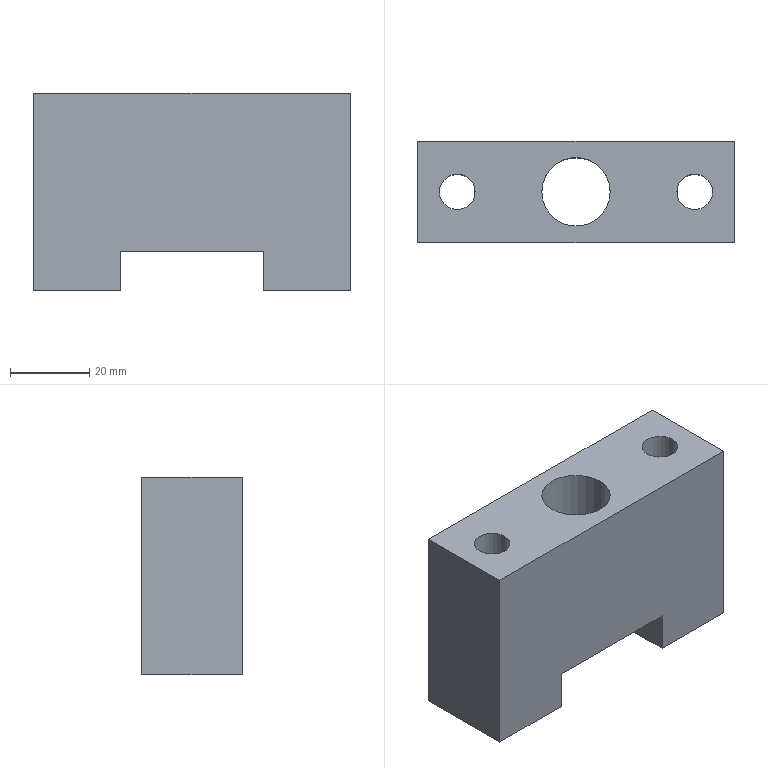Part | STEP file | giu lo xo day chot xien | 1 solid | 16 faces | box 80 x 25.5 x 50 mm | volume 77062 mm3 | plane 10 | cylinder 6 | commonest cylinder face diameters 9 x4 17.294 x2
STEP:
#1=CARTESIAN_POINT('',(0.,0.,0.));
#2=DIRECTION('',(0.,0.,1.));
#3=DIRECTION('',(1.,0.,0.));
#4=AXIS2_PLACEMENT_3D('',#1,#2,#3);
#5=CARTESIAN_POINT('',(14.5,12.75,0.));
#6=VERTEX_POINT('',#5);
#7=CARTESIAN_POINT('',(14.5,12.75,50.));
#8=VERTEX_POINT('',#7);
#9=CARTESIAN_POINT('',(14.5,12.75,-47.725));
#10=DIRECTION('',(0.,0.,1.));
#11=VECTOR('',#10,1.);
#12=LINE('',#9,#11);
#13=CARTESIAN_POINT('',(10.,12.75,-47.725));
#14=DIRECTION('',(0.,0.,1.));
#15=DIRECTION('',(1.,0.,0.));
#16=AXIS2_PLACEMENT_3D('',#13,#14,#15);
#17=CYLINDRICAL_SURFACE('',#16,4.5);
#18=CARTESIAN_POINT('',(6.283,0.));
#19=DIRECTION('',(0.,1.));
#20=VECTOR('',#19,1.);
#21=LINE('',#18,#20);
#22=(GEOMETRIC_REPRESENTATION_CONTEXT(2)PARAMETRIC_REPRESENTATION_CONTEXT()REPRESENTATION_CONTEXT('',''));
#23=DEFINITIONAL_REPRESENTATION('',(#21),#22);
#24=PCURVE('',#17,#23);
#25=CARTESIAN_POINT('',(10.,12.75,-47.725));
#26=DIRECTION('',(0.,0.,1.));
#27=DIRECTION('',(1.,0.,0.));
#28=AXIS2_PLACEMENT_3D('',#25,#26,#27);
#29=CYLINDRICAL_SURFACE('',#28,4.5);
#30=CARTESIAN_POINT('',(0.,0.));
#31=DIRECTION('',(0.,1.));
#32=VECTOR('',#31,1.);
#33=LINE('',#30,#32);
#34=(GEOMETRIC_REPRESENTATION_CONTEXT(2)PARAMETRIC_REPRESENTATION_CONTEXT()REPRESENTATION_CONTEXT('',''));
#35=DEFINITIONAL_REPRESENTATION('',(#33),#34);
#36=PCURVE('',#29,#35);
#37=SURFACE_CURVE('',#12,(#24,#36),.PCURVE_S1.);
#38=EDGE_CURVE('',#6,#8,#37,.T.);
#39=ORIENTED_EDGE('',*,*,#38,.T.);
#40=CARTESIAN_POINT('',(5.5,12.75,50.));
#41=VERTEX_POINT('',#40);
#42=CARTESIAN_POINT('',(10.,12.75,50.));
#43=DIRECTION('',(0.,0.,-1.));
#44=DIRECTION('',(1.,0.,0.));
#45=AXIS2_PLACEMENT_3D('',#42,#43,#44);
#46=CIRCLE('',#45,4.5);
#47=CARTESIAN_POINT('',(6.283,97.725));
#48=DIRECTION('',(-1.,0.));
#49=VECTOR('',#48,1.);
#50=LINE('',#47,#49);
#51=(GEOMETRIC_REPRESENTATION_CONTEXT(2)PARAMETRIC_REPRESENTATION_CONTEXT()REPRESENTATION_CONTEXT('',''));
#52=DEFINITIONAL_REPRESENTATION('',(#50),#51);
#53=PCURVE('',#17,#52);
#54=CARTESIAN_POINT('',(40.,12.75,50.));
#55=DIRECTION('',(0.,0.,1.));
#56=DIRECTION('',(1.,0.,0.));
#57=AXIS2_PLACEMENT_3D('',#54,#55,#56);
#58=PLANE('',#57);
#59=CARTESIAN_POINT('',(-25.5,0.));
#60=CARTESIAN_POINT('',(-25.5,-7.794));
#61=CARTESIAN_POINT('',(-32.25,-3.897));
#62=CARTESIAN_POINT('',(-39.,0.));
#63=CARTESIAN_POINT('',(-32.25,3.897));
#64=CARTESIAN_POINT('',(-25.5,7.794));
#65=CARTESIAN_POINT('',(-25.5,0.));
#66=(BOUNDED_CURVE()B_SPLINE_CURVE(2,(#59,#60,#61,#62,#63,#64,#65),.UNSPECIFIED.,.T.,.F.)B_SPLINE_CURVE_WITH_KNOTS((1,2,2,2,2,1),(-2.094,0.,2.094,4.189,6.283,8.378),.UNSPECIFIED.)CURVE()GEOMETRIC_REPRESENTATION_ITEM()RATIONAL_B_SPLINE_CURVE((1.,0.5,1.,0.5,1.,0.5,1.))REPRESENTATION_ITEM(''));
#67=(GEOMETRIC_REPRESENTATION_CONTEXT(2)PARAMETRIC_REPRESENTATION_CONTEXT()REPRESENTATION_CONTEXT('',''));
#68=DEFINITIONAL_REPRESENTATION('',(#66),#67);
#69=PCURVE('',#58,#68);
#70=SURFACE_CURVE('',#46,(#53,#69),.PCURVE_S1.);
#71=EDGE_CURVE('',#8,#41,#70,.T.);
#72=ORIENTED_EDGE('',*,*,#71,.T.);
#73=CARTESIAN_POINT('',(5.5,12.75,0.));
#74=VERTEX_POINT('',#73);
#75=CARTESIAN_POINT('',(5.5,12.75,-47.725));
#76=DIRECTION('',(0.,0.,1.));
#77=VECTOR('',#76,1.);
#78=LINE('',#75,#77);
#79=CARTESIAN_POINT('',(3.142,0.));
#80=DIRECTION('',(0.,1.));
#81=VECTOR('',#80,1.);
#82=LINE('',#79,#81);
#83=(GEOMETRIC_REPRESENTATION_CONTEXT(2)PARAMETRIC_REPRESENTATION_CONTEXT()REPRESENTATION_CONTEXT('',''));
#84=DEFINITIONAL_REPRESENTATION('',(#82),#83);
#85=PCURVE('',#17,#84);
#86=CARTESIAN_POINT('',(3.142,0.));
#87=DIRECTION('',(0.,1.));
#88=VECTOR('',#87,1.);
#89=LINE('',#86,#88);
#90=(GEOMETRIC_REPRESENTATION_CONTEXT(2)PARAMETRIC_REPRESENTATION_CONTEXT()REPRESENTATION_CONTEXT('',''));
#91=DEFINITIONAL_REPRESENTATION('',(#89),#90);
#92=PCURVE('',#29,#91);
#93=SURFACE_CURVE('',#78,(#85,#92),.PCURVE_S1.);
#94=EDGE_CURVE('',#74,#41,#93,.T.);
#95=ORIENTED_EDGE('',*,*,#94,.F.);
#96=CARTESIAN_POINT('',(10.,12.75,0.));
#97=DIRECTION('',(0.,0.,-1.));
#98=DIRECTION('',(1.,0.,0.));
#99=AXIS2_PLACEMENT_3D('',#96,#97,#98);
#100=CIRCLE('',#99,4.5);
#101=CARTESIAN_POINT('',(6.283,47.725));
#102=DIRECTION('',(-1.,0.));
#103=VECTOR('',#102,1.);
#104=LINE('',#101,#103);
#105=(GEOMETRIC_REPRESENTATION_CONTEXT(2)PARAMETRIC_REPRESENTATION_CONTEXT()REPRESENTATION_CONTEXT('',''));
#106=DEFINITIONAL_REPRESENTATION('',(#104),#105);
#107=PCURVE('',#17,#106);
#108=CARTESIAN_POINT('',(40.,12.75,0.));
#109=DIRECTION('',(0.,0.,1.));
#110=DIRECTION('',(1.,0.,0.));
#111=AXIS2_PLACEMENT_3D('',#108,#109,#110);
#112=PLANE('',#111);
#113=CARTESIAN_POINT('',(-25.5,0.));
#114=CARTESIAN_POINT('',(-25.5,-7.794));
#115=CARTESIAN_POINT('',(-32.25,-3.897));
#116=CARTESIAN_POINT('',(-39.,0.));
#117=CARTESIAN_POINT('',(-32.25,3.897));
#118=CARTESIAN_POINT('',(-25.5,7.794));
#119=CARTESIAN_POINT('',(-25.5,0.));
#120=(BOUNDED_CURVE()B_SPLINE_CURVE(2,(#113,#114,#115,#116,#117,#118,#119),.UNSPECIFIED.,.T.,.F.)B_SPLINE_CURVE_WITH_KNOTS((1,2,2,2,2,1),(-2.094,0.,2.094,4.189,6.283,8.378),.UNSPECIFIED.)CURVE()GEOMETRIC_REPRESENTATION_ITEM()RATIONAL_B_SPLINE_CURVE((1.,0.5,1.,0.5,1.,0.5,1.))REPRESENTATION_ITEM(''));
#121=(GEOMETRIC_REPRESENTATION_CONTEXT(2)PARAMETRIC_REPRESENTATION_CONTEXT()REPRESENTATION_CONTEXT('',''));
#122=DEFINITIONAL_REPRESENTATION('',(#120),#121);
#123=PCURVE('',#112,#122);
#124=SURFACE_CURVE('',#100,(#107,#123),.PCURVE_S1.);
#125=EDGE_CURVE('',#6,#74,#124,.T.);
#126=ORIENTED_EDGE('',*,*,#125,.F.);
#127=EDGE_LOOP('',(#39,#72,#95,#126));
#128=FACE_BOUND('',#127,.F.);
#129=ADVANCED_FACE('',(#128),#17,.F.);
#130=CARTESIAN_POINT('',(74.5,12.75,0.));
#131=VERTEX_POINT('',#130);
#132=CARTESIAN_POINT('',(74.5,12.75,50.));
#133=VERTEX_POINT('',#132);
#134=CARTESIAN_POINT('',(74.5,12.75,-47.725));
#135=DIRECTION('',(0.,0.,1.));
#136=VECTOR('',#135,1.);
#137=LINE('',#134,#136);
#138=CARTESIAN_POINT('',(70.,12.75,-47.725));
#139=DIRECTION('',(0.,0.,1.));
#140=DIRECTION('',(1.,0.,0.));
#141=AXIS2_PLACEMENT_3D('',#138,#139,#140);
#142=CYLINDRICAL_SURFACE('',#141,4.5);
#143=CARTESIAN_POINT('',(6.283,0.));
#144=DIRECTION('',(0.,1.));
#145=VECTOR('',#144,1.);
#146=LINE('',#143,#145);
#147=(GEOMETRIC_REPRESENTATION_CONTEXT(2)PARAMETRIC_REPRESENTATION_CONTEXT()REPRESENTATION_CONTEXT('',''));
#148=DEFINITIONAL_REPRESENTATION('',(#146),#147);
#149=PCURVE('',#142,#148);
#150=CARTESIAN_POINT('',(70.,12.75,-47.725));
#151=DIRECTION('',(0.,0.,1.));
#152=DIRECTION('',(1.,0.,0.));
#153=AXIS2_PLACEMENT_3D('',#150,#151,#152);
#154=CYLINDRICAL_SURFACE('',#153,4.5);
#155=CARTESIAN_POINT('',(0.,0.));
#156=DIRECTION('',(0.,1.));
#157=VECTOR('',#156,1.);
#158=LINE('',#155,#157);
#159=(GEOMETRIC_REPRESENTATION_CONTEXT(2)PARAMETRIC_REPRESENTATION_CONTEXT()REPRESENTATION_CONTEXT('',''));
#160=DEFINITIONAL_REPRESENTATION('',(#158),#159);
#161=PCURVE('',#154,#160);
#162=SURFACE_CURVE('',#137,(#149,#161),.PCURVE_S1.);
#163=EDGE_CURVE('',#131,#133,#162,.T.);
#164=ORIENTED_EDGE('',*,*,#163,.T.);
#165=CARTESIAN_POINT('',(65.5,12.75,50.));
#166=VERTEX_POINT('',#165);
#167=CARTESIAN_POINT('',(70.,12.75,50.));
#168=DIRECTION('',(0.,0.,-1.));
#169=DIRECTION('',(1.,0.,0.));
#170=AXIS2_PLACEMENT_3D('',#167,#168,#169);
#171=CIRCLE('',#170,4.5);
#172=CARTESIAN_POINT('',(6.283,97.725));
#173=DIRECTION('',(-1.,0.));
#174=VECTOR('',#173,1.);
#175=LINE('',#172,#174);
#176=(GEOMETRIC_REPRESENTATION_CONTEXT(2)PARAMETRIC_REPRESENTATION_CONTEXT()REPRESENTATION_CONTEXT('',''));
#177=DEFINITIONAL_REPRESENTATION('',(#175),#176);
#178=PCURVE('',#142,#177);
#179=CARTESIAN_POINT('',(34.5,0.));
#180=CARTESIAN_POINT('',(34.5,-7.794));
#181=CARTESIAN_POINT('',(27.75,-3.897));
#182=CARTESIAN_POINT('',(21.,0.));
#183=CARTESIAN_POINT('',(27.75,3.897));
#184=CARTESIAN_POINT('',(34.5,7.794));
#185=CARTESIAN_POINT('',(34.5,0.));
#186=(BOUNDED_CURVE()B_SPLINE_CURVE(2,(#179,#180,#181,#182,#183,#184,#185),.UNSPECIFIED.,.T.,.F.)B_SPLINE_CURVE_WITH_KNOTS((1,2,2,2,2,1),(-2.094,0.,2.094,4.189,6.283,8.378),.UNSPECIFIED.)CURVE()GEOMETRIC_REPRESENTATION_ITEM()RATIONAL_B_SPLINE_CURVE((1.,0.5,1.,0.5,1.,0.5,1.))REPRESENTATION_ITEM(''));
#187=(GEOMETRIC_REPRESENTATION_CONTEXT(2)PARAMETRIC_REPRESENTATION_CONTEXT()REPRESENTATION_CONTEXT('',''));
#188=DEFINITIONAL_REPRESENTATION('',(#186),#187);
#189=PCURVE('',#58,#188);
#190=SURFACE_CURVE('',#171,(#178,#189),.PCURVE_S1.);
#191=EDGE_CURVE('',#133,#166,#190,.T.);
#192=ORIENTED_EDGE('',*,*,#191,.T.);
#193=CARTESIAN_POINT('',(65.5,12.75,0.));
#194=VERTEX_POINT('',#193);
#195=CARTESIAN_POINT('',(65.5,12.75,-47.725));
#196=DIRECTION('',(0.,0.,1.));
#197=VECTOR('',#196,1.);
#198=LINE('',#195,#197);
#199=CARTESIAN_POINT('',(3.142,0.));
#200=DIRECTION('',(0.,1.));
#201=VECTOR('',#200,1.);
#202=LINE('',#199,#201);
#203=(GEOMETRIC_REPRESENTATION_CONTEXT(2)PARAMETRIC_REPRESENTATION_CONTEXT()REPRESENTATION_CONTEXT('',''));
#204=DEFINITIONAL_REPRESENTATION('',(#202),#203);
#205=PCURVE('',#142,#204);
#206=CARTESIAN_POINT('',(3.142,0.));
#207=DIRECTION('',(0.,1.));
#208=VECTOR('',#207,1.);
#209=LINE('',#206,#208);
#210=(GEOMETRIC_REPRESENTATION_CONTEXT(2)PARAMETRIC_REPRESENTATION_CONTEXT()REPRESENTATION_CONTEXT('',''));
#211=DEFINITIONAL_REPRESENTATION('',(#209),#210);
#212=PCURVE('',#154,#211);
#213=SURFACE_CURVE('',#198,(#205,#212),.PCURVE_S1.);
#214=EDGE_CURVE('',#194,#166,#213,.T.);
#215=ORIENTED_EDGE('',*,*,#214,.F.);
#216=CARTESIAN_POINT('',(70.,12.75,0.));
#217=DIRECTION('',(0.,0.,-1.));
#218=DIRECTION('',(1.,0.,0.));
#219=AXIS2_PLACEMENT_3D('',#216,#217,#218);
#220=CIRCLE('',#219,4.5);
#221=CARTESIAN_POINT('',(6.283,47.725));
#222=DIRECTION('',(-1.,0.));
#223=VECTOR('',#222,1.);
#224=LINE('',#221,#223);
#225=(GEOMETRIC_REPRESENTATION_CONTEXT(2)PARAMETRIC_REPRESENTATION_CONTEXT()REPRESENTATION_CONTEXT('',''));
#226=DEFINITIONAL_REPRESENTATION('',(#224),#225);
#227=PCURVE('',#142,#226);
#228=CARTESIAN_POINT('',(40.,12.75,0.));
#229=DIRECTION('',(0.,0.,1.));
#230=DIRECTION('',(1.,0.,0.));
#231=AXIS2_PLACEMENT_3D('',#228,#229,#230);
#232=PLANE('',#231);
#233=CARTESIAN_POINT('',(34.5,0.));
#234=CARTESIAN_POINT('',(34.5,-7.794));
#235=CARTESIAN_POINT('',(27.75,-3.897));
#236=CARTESIAN_POINT('',(21.,0.));
#237=CARTESIAN_POINT('',(27.75,3.897));
#238=CARTESIAN_POINT('',(34.5,7.794));
#239=CARTESIAN_POINT('',(34.5,0.));
#240=(BOUNDED_CURVE()B_SPLINE_CURVE(2,(#233,#234,#235,#236,#237,#238,#239),.UNSPECIFIED.,.T.,.F.)B_SPLINE_CURVE_WITH_KNOTS((1,2,2,2,2,1),(-2.094,0.,2.094,4.189,6.283,8.378),.UNSPECIFIED.)CURVE()GEOMETRIC_REPRESENTATION_ITEM()RATIONAL_B_SPLINE_CURVE((1.,0.5,1.,0.5,1.,0.5,1.))REPRESENTATION_ITEM(''));
#241=(GEOMETRIC_REPRESENTATION_CONTEXT(2)PARAMETRIC_REPRESENTATION_CONTEXT()REPRESENTATION_CONTEXT('',''));
#242=DEFINITIONAL_REPRESENTATION('',(#240),#241);
#243=PCURVE('',#232,#242);
#244=SURFACE_CURVE('',#220,(#227,#243),.PCURVE_S1.);
#245=EDGE_CURVE('',#131,#194,#244,.T.);
#246=ORIENTED_EDGE('',*,*,#245,.F.);
#247=EDGE_LOOP('',(#164,#192,#215,#246));
#248=FACE_BOUND('',#247,.F.);
#249=ADVANCED_FACE('',(#248),#142,.F.);
#250=CARTESIAN_POINT('',(48.647,12.75,10.));
#251=VERTEX_POINT('',#250);
#252=CARTESIAN_POINT('',(48.647,12.75,50.));
#253=VERTEX_POINT('',#252);
#254=CARTESIAN_POINT('',(48.647,12.75,-47.725));
#255=DIRECTION('',(0.,0.,1.));
#256=VECTOR('',#255,1.);
#257=LINE('',#254,#256);
#258=CARTESIAN_POINT('',(40.,12.75,-47.725));
#259=DIRECTION('',(0.,0.,1.));
#260=DIRECTION('',(1.,0.,0.));
#261=AXIS2_PLACEMENT_3D('',#258,#259,#260);
#262=CYLINDRICAL_SURFACE('',#261,8.647);
#263=CARTESIAN_POINT('',(6.283,0.));
#264=DIRECTION('',(0.,1.));
#265=VECTOR('',#264,1.);
#266=LINE('',#263,#265);
#267=(GEOMETRIC_REPRESENTATION_CONTEXT(2)PARAMETRIC_REPRESENTATION_CONTEXT()REPRESENTATION_CONTEXT('',''));
#268=DEFINITIONAL_REPRESENTATION('',(#266),#267);
#269=PCURVE('',#262,#268);
#270=CARTESIAN_POINT('',(40.,12.75,-47.725));
#271=DIRECTION('',(0.,0.,1.));
#272=DIRECTION('',(1.,0.,0.));
#273=AXIS2_PLACEMENT_3D('',#270,#271,#272);
#274=CYLINDRICAL_SURFACE('',#273,8.647);
#275=CARTESIAN_POINT('',(0.,0.));
#276=DIRECTION('',(0.,1.));
#277=VECTOR('',#276,1.);
#278=LINE('',#275,#277);
#279=(GEOMETRIC_REPRESENTATION_CONTEXT(2)PARAMETRIC_REPRESENTATION_CONTEXT()REPRESENTATION_CONTEXT('',''));
#280=DEFINITIONAL_REPRESENTATION('',(#278),#279);
#281=PCURVE('',#274,#280);
#282=SURFACE_CURVE('',#257,(#269,#281),.PCURVE_S1.);
#283=EDGE_CURVE('',#251,#253,#282,.T.);
#284=ORIENTED_EDGE('',*,*,#283,.T.);
#285=CARTESIAN_POINT('',(31.353,12.75,50.));
#286=VERTEX_POINT('',#285);
#287=CARTESIAN_POINT('',(40.,12.75,50.));
#288=DIRECTION('',(0.,0.,-1.));
#289=DIRECTION('',(1.,0.,0.));
#290=AXIS2_PLACEMENT_3D('',#287,#288,#289);
#291=CIRCLE('',#290,8.647);
#292=CARTESIAN_POINT('',(6.283,97.725));
#293=DIRECTION('',(-1.,0.));
#294=VECTOR('',#293,1.);
#295=LINE('',#292,#294);
#296=(GEOMETRIC_REPRESENTATION_CONTEXT(2)PARAMETRIC_REPRESENTATION_CONTEXT()REPRESENTATION_CONTEXT('',''));
#297=DEFINITIONAL_REPRESENTATION('',(#295),#296);
#298=PCURVE('',#262,#297);
#299=CARTESIAN_POINT('',(8.647,0.));
#300=CARTESIAN_POINT('',(8.647,-14.977));
#301=CARTESIAN_POINT('',(-4.324,-7.489));
#302=CARTESIAN_POINT('',(-17.294,0.));
#303=CARTESIAN_POINT('',(-4.324,7.489));
#304=CARTESIAN_POINT('',(8.647,14.977));
#305=CARTESIAN_POINT('',(8.647,0.));
#306=(BOUNDED_CURVE()B_SPLINE_CURVE(2,(#299,#300,#301,#302,#303,#304,#305),.UNSPECIFIED.,.T.,.F.)B_SPLINE_CURVE_WITH_KNOTS((1,2,2,2,2,1),(-2.094,0.,2.094,4.189,6.283,8.378),.UNSPECIFIED.)CURVE()GEOMETRIC_REPRESENTATION_ITEM()RATIONAL_B_SPLINE_CURVE((1.,0.5,1.,0.5,1.,0.5,1.))REPRESENTATION_ITEM(''));
#307=(GEOMETRIC_REPRESENTATION_CONTEXT(2)PARAMETRIC_REPRESENTATION_CONTEXT()REPRESENTATION_CONTEXT('',''));
#308=DEFINITIONAL_REPRESENTATION('',(#306),#307);
#309=PCURVE('',#58,#308);
#310=SURFACE_CURVE('',#291,(#298,#309),.PCURVE_S1.);
#311=EDGE_CURVE('',#253,#286,#310,.T.);
#312=ORIENTED_EDGE('',*,*,#311,.T.);
#313=CARTESIAN_POINT('',(31.353,12.75,10.));
#314=VERTEX_POINT('',#313);
#315=CARTESIAN_POINT('',(31.353,12.75,-47.725));
#316=DIRECTION('',(0.,0.,1.));
#317=VECTOR('',#316,1.);
#318=LINE('',#315,#317);
#319=CARTESIAN_POINT('',(3.142,0.));
#320=DIRECTION('',(0.,1.));
#321=VECTOR('',#320,1.);
#322=LINE('',#319,#321);
#323=(GEOMETRIC_REPRESENTATION_CONTEXT(2)PARAMETRIC_REPRESENTATION_CONTEXT()REPRESENTATION_CONTEXT('',''));
#324=DEFINITIONAL_REPRESENTATION('',(#322),#323);
#325=PCURVE('',#262,#324);
#326=CARTESIAN_POINT('',(3.142,0.));
#327=DIRECTION('',(0.,1.));
#328=VECTOR('',#327,1.);
#329=LINE('',#326,#328);
#330=(GEOMETRIC_REPRESENTATION_CONTEXT(2)PARAMETRIC_REPRESENTATION_CONTEXT()REPRESENTATION_CONTEXT('',''));
#331=DEFINITIONAL_REPRESENTATION('',(#329),#330);
#332=PCURVE('',#274,#331);
#333=SURFACE_CURVE('',#318,(#325,#332),.PCURVE_S1.);
#334=EDGE_CURVE('',#314,#286,#333,.T.);
#335=ORIENTED_EDGE('',*,*,#334,.F.);
#336=CARTESIAN_POINT('',(40.,12.75,10.));
#337=DIRECTION('',(0.,0.,-1.));
#338=DIRECTION('',(1.,0.,0.));
#339=AXIS2_PLACEMENT_3D('',#336,#337,#338);
#340=CIRCLE('',#339,8.647);
#341=CARTESIAN_POINT('',(6.283,57.725));
#342=DIRECTION('',(-1.,0.));
#343=VECTOR('',#342,1.);
#344=LINE('',#341,#343);
#345=(GEOMETRIC_REPRESENTATION_CONTEXT(2)PARAMETRIC_REPRESENTATION_CONTEXT()REPRESENTATION_CONTEXT('',''));
#346=DEFINITIONAL_REPRESENTATION('',(#344),#345);
#347=PCURVE('',#262,#346);
#348=CARTESIAN_POINT('',(40.,12.75,10.));
#349=DIRECTION('',(0.,0.,1.));
#350=DIRECTION('',(1.,0.,0.));
#351=AXIS2_PLACEMENT_3D('',#348,#349,#350);
#352=PLANE('',#351);
#353=CARTESIAN_POINT('',(8.647,0.));
#354=CARTESIAN_POINT('',(8.647,-14.977));
#355=CARTESIAN_POINT('',(-4.324,-7.489));
#356=CARTESIAN_POINT('',(-17.294,0.));
#357=CARTESIAN_POINT('',(-4.324,7.489));
#358=CARTESIAN_POINT('',(8.647,14.977));
#359=CARTESIAN_POINT('',(8.647,0.));
#360=(BOUNDED_CURVE()B_SPLINE_CURVE(2,(#353,#354,#355,#356,#357,#358,#359),.UNSPECIFIED.,.T.,.F.)B_SPLINE_CURVE_WITH_KNOTS((1,2,2,2,2,1),(-2.094,0.,2.094,4.189,6.283,8.378),.UNSPECIFIED.)CURVE()GEOMETRIC_REPRESENTATION_ITEM()RATIONAL_B_SPLINE_CURVE((1.,0.5,1.,0.5,1.,0.5,1.))REPRESENTATION_ITEM(''));
#361=(GEOMETRIC_REPRESENTATION_CONTEXT(2)PARAMETRIC_REPRESENTATION_CONTEXT()REPRESENTATION_CONTEXT('',''));
#362=DEFINITIONAL_REPRESENTATION('',(#360),#361);
#363=PCURVE('',#352,#362);
#364=SURFACE_CURVE('',#340,(#347,#363),.PCURVE_S1.);
#365=EDGE_CURVE('',#251,#314,#364,.T.);
#366=ORIENTED_EDGE('',*,*,#365,.F.);
#367=EDGE_LOOP('',(#284,#312,#335,#366));
#368=FACE_BOUND('',#367,.F.);
#369=ADVANCED_FACE('',(#368),#262,.F.);
#370=CARTESIAN_POINT('',(0.,0.,50.));
#371=VERTEX_POINT('',#370);
#372=CARTESIAN_POINT('',(0.,0.,0.));
#373=VERTEX_POINT('',#372);
#374=CARTESIAN_POINT('',(0.,0.,0.));
#375=DIRECTION('',(0.,0.,-1.));
#376=VECTOR('',#375,1.);
#377=LINE('',#374,#376);
#378=CARTESIAN_POINT('',(80.,0.,0.));
#379=DIRECTION('',(0.,-1.,0.));
#380=DIRECTION('',(0.,0.,-1.));
#381=AXIS2_PLACEMENT_3D('',#378,#379,#380);
#382=PLANE('',#381);
#383=CARTESIAN_POINT('',(0.,-80.));
#384=DIRECTION('',(1.,0.));
#385=VECTOR('',#384,1.);
#386=LINE('',#383,#385);
#387=(GEOMETRIC_REPRESENTATION_CONTEXT(2)PARAMETRIC_REPRESENTATION_CONTEXT()REPRESENTATION_CONTEXT('',''));
#388=DEFINITIONAL_REPRESENTATION('',(#386),#387);
#389=PCURVE('',#382,#388);
#390=CARTESIAN_POINT('',(0.,0.,0.));
#391=DIRECTION('',(-1.,0.,0.));
#392=DIRECTION('',(0.,0.,1.));
#393=AXIS2_PLACEMENT_3D('',#390,#391,#392);
#394=PLANE('',#393);
#395=CARTESIAN_POINT('',(0.,0.));
#396=DIRECTION('',(-1.,0.));
#397=VECTOR('',#396,1.);
#398=LINE('',#395,#397);
#399=(GEOMETRIC_REPRESENTATION_CONTEXT(2)PARAMETRIC_REPRESENTATION_CONTEXT()REPRESENTATION_CONTEXT('',''));
#400=DEFINITIONAL_REPRESENTATION('',(#398),#399);
#401=PCURVE('',#394,#400);
#402=SURFACE_CURVE('',#377,(#389,#401),.PCURVE_S1.);
#403=EDGE_CURVE('',#371,#373,#402,.T.);
#404=ORIENTED_EDGE('',*,*,#403,.T.);
#405=CARTESIAN_POINT('',(22.,0.,0.));
#406=VERTEX_POINT('',#405);
#407=CARTESIAN_POINT('',(80.,0.,0.));
#408=DIRECTION('',(1.,0.,0.));
#409=VECTOR('',#408,1.);
#410=LINE('',#407,#409);
#411=CARTESIAN_POINT('',(0.,0.));
#412=DIRECTION('',(0.,1.));
#413=VECTOR('',#412,1.);
#414=LINE('',#411,#413);
#415=(GEOMETRIC_REPRESENTATION_CONTEXT(2)PARAMETRIC_REPRESENTATION_CONTEXT()REPRESENTATION_CONTEXT('',''));
#416=DEFINITIONAL_REPRESENTATION('',(#414),#415);
#417=PCURVE('',#382,#416);
#418=CARTESIAN_POINT('',(40.,-12.75));
#419=DIRECTION('',(1.,0.));
#420=VECTOR('',#419,1.);
#421=LINE('',#418,#420);
#422=(GEOMETRIC_REPRESENTATION_CONTEXT(2)PARAMETRIC_REPRESENTATION_CONTEXT()REPRESENTATION_CONTEXT('',''));
#423=DEFINITIONAL_REPRESENTATION('',(#421),#422);
#424=PCURVE('',#112,#423);
#425=SURFACE_CURVE('',#410,(#417,#424),.PCURVE_S1.);
#426=EDGE_CURVE('',#373,#406,#425,.T.);
#427=ORIENTED_EDGE('',*,*,#426,.T.);
#428=CARTESIAN_POINT('',(22.,0.,10.));
#429=VERTEX_POINT('',#428);
#430=CARTESIAN_POINT('',(22.,0.,0.));
#431=DIRECTION('',(0.,0.,1.));
#432=VECTOR('',#431,1.);
#433=LINE('',#430,#432);
#434=CARTESIAN_POINT('',(0.,-58.));
#435=DIRECTION('',(-1.,0.));
#436=VECTOR('',#435,1.);
#437=LINE('',#434,#436);
#438=(GEOMETRIC_REPRESENTATION_CONTEXT(2)PARAMETRIC_REPRESENTATION_CONTEXT()REPRESENTATION_CONTEXT('',''));
#439=DEFINITIONAL_REPRESENTATION('',(#437),#438);
#440=PCURVE('',#382,#439);
#441=CARTESIAN_POINT('',(22.,0.,0.));
#442=DIRECTION('',(-1.,0.,0.));
#443=DIRECTION('',(0.,0.,1.));
#444=AXIS2_PLACEMENT_3D('',#441,#442,#443);
#445=PLANE('',#444);
#446=CARTESIAN_POINT('',(0.,0.));
#447=DIRECTION('',(1.,0.));
#448=VECTOR('',#447,1.);
#449=LINE('',#446,#448);
#450=(GEOMETRIC_REPRESENTATION_CONTEXT(2)PARAMETRIC_REPRESENTATION_CONTEXT()REPRESENTATION_CONTEXT('',''));
#451=DEFINITIONAL_REPRESENTATION('',(#449),#450);
#452=PCURVE('',#445,#451);
#453=SURFACE_CURVE('',#433,(#440,#452),.PCURVE_S1.);
#454=EDGE_CURVE('',#406,#429,#453,.T.);
#455=ORIENTED_EDGE('',*,*,#454,.T.);
#456=CARTESIAN_POINT('',(58.,0.,10.));
#457=VERTEX_POINT('',#456);
#458=CARTESIAN_POINT('',(80.,0.,10.));
#459=DIRECTION('',(1.,0.,0.));
#460=VECTOR('',#459,1.);
#461=LINE('',#458,#460);
#462=CARTESIAN_POINT('',(-10.,0.));
#463=DIRECTION('',(0.,1.));
#464=VECTOR('',#463,1.);
#465=LINE('',#462,#464);
#466=(GEOMETRIC_REPRESENTATION_CONTEXT(2)PARAMETRIC_REPRESENTATION_CONTEXT()REPRESENTATION_CONTEXT('',''));
#467=DEFINITIONAL_REPRESENTATION('',(#465),#466);
#468=PCURVE('',#382,#467);
#469=CARTESIAN_POINT('',(40.,-12.75));
#470=DIRECTION('',(1.,0.));
#471=VECTOR('',#470,1.);
#472=LINE('',#469,#471);
#473=(GEOMETRIC_REPRESENTATION_CONTEXT(2)PARAMETRIC_REPRESENTATION_CONTEXT()REPRESENTATION_CONTEXT('',''));
#474=DEFINITIONAL_REPRESENTATION('',(#472),#473);
#475=PCURVE('',#352,#474);
#476=SURFACE_CURVE('',#461,(#468,#475),.PCURVE_S1.);
#477=EDGE_CURVE('',#429,#457,#476,.T.);
#478=ORIENTED_EDGE('',*,*,#477,.T.);
#479=CARTESIAN_POINT('',(58.,0.,0.));
#480=VERTEX_POINT('',#479);
#481=CARTESIAN_POINT('',(58.,0.,0.));
#482=DIRECTION('',(0.,0.,-1.));
#483=VECTOR('',#482,1.);
#484=LINE('',#481,#483);
#485=CARTESIAN_POINT('',(0.,-22.));
#486=DIRECTION('',(1.,0.));
#487=VECTOR('',#486,1.);
#488=LINE('',#485,#487);
#489=(GEOMETRIC_REPRESENTATION_CONTEXT(2)PARAMETRIC_REPRESENTATION_CONTEXT()REPRESENTATION_CONTEXT('',''));
#490=DEFINITIONAL_REPRESENTATION('',(#488),#489);
#491=PCURVE('',#382,#490);
#492=CARTESIAN_POINT('',(58.,25.5,0.));
#493=DIRECTION('',(1.,0.,0.));
#494=DIRECTION('',(0.,0.,-1.));
#495=AXIS2_PLACEMENT_3D('',#492,#493,#494);
#496=PLANE('',#495);
#497=CARTESIAN_POINT('',(0.,-25.5));
#498=DIRECTION('',(1.,0.));
#499=VECTOR('',#498,1.);
#500=LINE('',#497,#499);
#501=(GEOMETRIC_REPRESENTATION_CONTEXT(2)PARAMETRIC_REPRESENTATION_CONTEXT()REPRESENTATION_CONTEXT('',''));
#502=DEFINITIONAL_REPRESENTATION('',(#500),#501);
#503=PCURVE('',#496,#502);
#504=SURFACE_CURVE('',#484,(#491,#503),.PCURVE_S1.);
#505=EDGE_CURVE('',#457,#480,#504,.T.);
#506=ORIENTED_EDGE('',*,*,#505,.T.);
#507=CARTESIAN_POINT('',(80.,0.,0.));
#508=VERTEX_POINT('',#507);
#509=CARTESIAN_POINT('',(80.,0.,0.));
#510=DIRECTION('',(1.,0.,0.));
#511=VECTOR('',#510,1.);
#512=LINE('',#509,#511);
#513=CARTESIAN_POINT('',(0.,0.));
#514=DIRECTION('',(0.,1.));
#515=VECTOR('',#514,1.);
#516=LINE('',#513,#515);
#517=(GEOMETRIC_REPRESENTATION_CONTEXT(2)PARAMETRIC_REPRESENTATION_CONTEXT()REPRESENTATION_CONTEXT('',''));
#518=DEFINITIONAL_REPRESENTATION('',(#516),#517);
#519=PCURVE('',#382,#518);
#520=CARTESIAN_POINT('',(40.,-12.75));
#521=DIRECTION('',(1.,0.));
#522=VECTOR('',#521,1.);
#523=LINE('',#520,#522);
#524=(GEOMETRIC_REPRESENTATION_CONTEXT(2)PARAMETRIC_REPRESENTATION_CONTEXT()REPRESENTATION_CONTEXT('',''));
#525=DEFINITIONAL_REPRESENTATION('',(#523),#524);
#526=PCURVE('',#232,#525);
#527=SURFACE_CURVE('',#512,(#519,#526),.PCURVE_S1.);
#528=EDGE_CURVE('',#480,#508,#527,.T.);
#529=ORIENTED_EDGE('',*,*,#528,.T.);
#530=CARTESIAN_POINT('',(80.,0.,50.));
#531=VERTEX_POINT('',#530);
#532=CARTESIAN_POINT('',(80.,0.,0.));
#533=DIRECTION('',(0.,0.,1.));
#534=VECTOR('',#533,1.);
#535=LINE('',#532,#534);
#536=CARTESIAN_POINT('',(0.,0.));
#537=DIRECTION('',(-1.,0.));
#538=VECTOR('',#537,1.);
#539=LINE('',#536,#538);
#540=(GEOMETRIC_REPRESENTATION_CONTEXT(2)PARAMETRIC_REPRESENTATION_CONTEXT()REPRESENTATION_CONTEXT('',''));
#541=DEFINITIONAL_REPRESENTATION('',(#539),#540);
#542=PCURVE('',#382,#541);
#543=CARTESIAN_POINT('',(80.,25.5,0.));
#544=DIRECTION('',(1.,0.,0.));
#545=DIRECTION('',(0.,0.,-1.));
#546=AXIS2_PLACEMENT_3D('',#543,#544,#545);
#547=PLANE('',#546);
#548=CARTESIAN_POINT('',(0.,-25.5));
#549=DIRECTION('',(-1.,0.));
#550=VECTOR('',#549,1.);
#551=LINE('',#548,#550);
#552=(GEOMETRIC_REPRESENTATION_CONTEXT(2)PARAMETRIC_REPRESENTATION_CONTEXT()REPRESENTATION_CONTEXT('',''));
#553=DEFINITIONAL_REPRESENTATION('',(#551),#552);
#554=PCURVE('',#547,#553);
#555=SURFACE_CURVE('',#535,(#542,#554),.PCURVE_S1.);
#556=EDGE_CURVE('',#508,#531,#555,.T.);
#557=ORIENTED_EDGE('',*,*,#556,.T.);
#558=CARTESIAN_POINT('',(80.,0.,50.));
#559=DIRECTION('',(-1.,0.,0.));
#560=VECTOR('',#559,1.);
#561=LINE('',#558,#560);
#562=CARTESIAN_POINT('',(-50.,0.));
#563=DIRECTION('',(0.,-1.));
#564=VECTOR('',#563,1.);
#565=LINE('',#562,#564);
#566=(GEOMETRIC_REPRESENTATION_CONTEXT(2)PARAMETRIC_REPRESENTATION_CONTEXT()REPRESENTATION_CONTEXT('',''));
#567=DEFINITIONAL_REPRESENTATION('',(#565),#566);
#568=PCURVE('',#382,#567);
#569=CARTESIAN_POINT('',(40.,-12.75));
#570=DIRECTION('',(-1.,0.));
#571=VECTOR('',#570,1.);
#572=LINE('',#569,#571);
#573=(GEOMETRIC_REPRESENTATION_CONTEXT(2)PARAMETRIC_REPRESENTATION_CONTEXT()REPRESENTATION_CONTEXT('',''));
#574=DEFINITIONAL_REPRESENTATION('',(#572),#573);
#575=PCURVE('',#58,#574);
#576=SURFACE_CURVE('',#561,(#568,#575),.PCURVE_S1.);
#577=EDGE_CURVE('',#531,#371,#576,.T.);
#578=ORIENTED_EDGE('',*,*,#577,.T.);
#579=EDGE_LOOP('',(#404,#427,#455,#478,#506,#529,#557,#578));
#580=FACE_BOUND('',#579,.T.);
#581=ADVANCED_FACE('',(#580),#382,.T.);
#582=ORIENTED_EDGE('',*,*,#125,.F.);
#583=CARTESIAN_POINT('',(10.,12.75,0.));
#584=DIRECTION('',(0.,0.,-1.));
#585=DIRECTION('',(1.,0.,0.));
#586=AXIS2_PLACEMENT_3D('',#583,#584,#585);
#587=CIRCLE('',#586,4.5);
#588=CARTESIAN_POINT('',(-25.5,0.));
#589=CARTESIAN_POINT('',(-25.5,-7.794));
#590=CARTESIAN_POINT('',(-32.25,-3.897));
#591=CARTESIAN_POINT('',(-39.,0.));
#592=CARTESIAN_POINT('',(-32.25,3.897));
#593=CARTESIAN_POINT('',(-25.5,7.794));
#594=CARTESIAN_POINT('',(-25.5,0.));
#595=(BOUNDED_CURVE()B_SPLINE_CURVE(2,(#588,#589,#590,#591,#592,#593,#594),.UNSPECIFIED.,.T.,.F.)B_SPLINE_CURVE_WITH_KNOTS((1,2,2,2,2,1),(-2.094,0.,2.094,4.189,6.283,8.378),.UNSPECIFIED.)CURVE()GEOMETRIC_REPRESENTATION_ITEM()RATIONAL_B_SPLINE_CURVE((1.,0.5,1.,0.5,1.,0.5,1.))REPRESENTATION_ITEM(''));
#596=(GEOMETRIC_REPRESENTATION_CONTEXT(2)PARAMETRIC_REPRESENTATION_CONTEXT()REPRESENTATION_CONTEXT('',''));
#597=DEFINITIONAL_REPRESENTATION('',(#595),#596);
#598=PCURVE('',#112,#597);
#599=CARTESIAN_POINT('',(6.283,47.725));
#600=DIRECTION('',(-1.,0.));
#601=VECTOR('',#600,1.);
#602=LINE('',#599,#601);
#603=(GEOMETRIC_REPRESENTATION_CONTEXT(2)PARAMETRIC_REPRESENTATION_CONTEXT()REPRESENTATION_CONTEXT('',''));
#604=DEFINITIONAL_REPRESENTATION('',(#602),#603);
#605=PCURVE('',#29,#604);
#606=SURFACE_CURVE('',#587,(#598,#605),.PCURVE_S1.);
#607=EDGE_CURVE('',#74,#6,#606,.T.);
#608=ORIENTED_EDGE('',*,*,#607,.F.);
#609=EDGE_LOOP('',(#582,#608));
#610=FACE_BOUND('',#609,.T.);
#611=ORIENTED_EDGE('',*,*,#426,.F.);
#612=CARTESIAN_POINT('',(0.,25.5,0.));
#613=VERTEX_POINT('',#612);
#614=CARTESIAN_POINT('',(0.,12.75,0.));
#615=DIRECTION('',(0.,-1.,0.));
#616=VECTOR('',#615,1.);
#617=LINE('',#614,#616);
#618=CARTESIAN_POINT('',(-40.,0.));
#619=DIRECTION('',(0.,-1.));
#620=VECTOR('',#619,1.);
#621=LINE('',#618,#620);
#622=(GEOMETRIC_REPRESENTATION_CONTEXT(2)PARAMETRIC_REPRESENTATION_CONTEXT()REPRESENTATION_CONTEXT('',''));
#623=DEFINITIONAL_REPRESENTATION('',(#621),#622);
#624=PCURVE('',#112,#623);
#625=CARTESIAN_POINT('',(0.,12.75));
#626=DIRECTION('',(0.,-1.));
#627=VECTOR('',#626,1.);
#628=LINE('',#625,#627);
#629=(GEOMETRIC_REPRESENTATION_CONTEXT(2)PARAMETRIC_REPRESENTATION_CONTEXT()REPRESENTATION_CONTEXT('',''));
#630=DEFINITIONAL_REPRESENTATION('',(#628),#629);
#631=PCURVE('',#394,#630);
#632=SURFACE_CURVE('',#617,(#624,#631),.PCURVE_S1.);
#633=EDGE_CURVE('',#613,#373,#632,.T.);
#634=ORIENTED_EDGE('',*,*,#633,.F.);
#635=CARTESIAN_POINT('',(22.,25.5,0.));
#636=VERTEX_POINT('',#635);
#637=CARTESIAN_POINT('',(40.,25.5,0.));
#638=DIRECTION('',(-1.,0.,0.));
#639=VECTOR('',#638,1.);
#640=LINE('',#637,#639);
#641=CARTESIAN_POINT('',(0.,12.75));
#642=DIRECTION('',(-1.,0.));
#643=VECTOR('',#642,1.);
#644=LINE('',#641,#643);
#645=(GEOMETRIC_REPRESENTATION_CONTEXT(2)PARAMETRIC_REPRESENTATION_CONTEXT()REPRESENTATION_CONTEXT('',''));
#646=DEFINITIONAL_REPRESENTATION('',(#644),#645);
#647=PCURVE('',#112,#646);
#648=CARTESIAN_POINT('',(0.,25.5,0.));
#649=DIRECTION('',(0.,1.,0.));
#650=DIRECTION('',(0.,0.,1.));
#651=AXIS2_PLACEMENT_3D('',#648,#649,#650);
#652=PLANE('',#651);
#653=CARTESIAN_POINT('',(0.,40.));
#654=DIRECTION('',(0.,-1.));
#655=VECTOR('',#654,1.);
#656=LINE('',#653,#655);
#657=(GEOMETRIC_REPRESENTATION_CONTEXT(2)PARAMETRIC_REPRESENTATION_CONTEXT()REPRESENTATION_CONTEXT('',''));
#658=DEFINITIONAL_REPRESENTATION('',(#656),#657);
#659=PCURVE('',#652,#658);
#660=SURFACE_CURVE('',#640,(#647,#659),.PCURVE_S1.);
#661=EDGE_CURVE('',#636,#613,#660,.T.);
#662=ORIENTED_EDGE('',*,*,#661,.F.);
#663=CARTESIAN_POINT('',(22.,12.75,0.));
#664=DIRECTION('',(0.,1.,0.));
#665=VECTOR('',#664,1.);
#666=LINE('',#663,#665);
#667=CARTESIAN_POINT('',(-18.,0.));
#668=DIRECTION('',(0.,1.));
#669=VECTOR('',#668,1.);
#670=LINE('',#667,#669);
#671=(GEOMETRIC_REPRESENTATION_CONTEXT(2)PARAMETRIC_REPRESENTATION_CONTEXT()REPRESENTATION_CONTEXT('',''));
#672=DEFINITIONAL_REPRESENTATION('',(#670),#671);
#673=PCURVE('',#112,#672);
#674=CARTESIAN_POINT('',(0.,12.75));
#675=DIRECTION('',(0.,1.));
#676=VECTOR('',#675,1.);
#677=LINE('',#674,#676);
#678=(GEOMETRIC_REPRESENTATION_CONTEXT(2)PARAMETRIC_REPRESENTATION_CONTEXT()REPRESENTATION_CONTEXT('',''));
#679=DEFINITIONAL_REPRESENTATION('',(#677),#678);
#680=PCURVE('',#445,#679);
#681=SURFACE_CURVE('',#666,(#673,#680),.PCURVE_S1.);
#682=EDGE_CURVE('',#406,#636,#681,.T.);
#683=ORIENTED_EDGE('',*,*,#682,.F.);
#684=EDGE_LOOP('',(#611,#634,#662,#683));
#685=FACE_BOUND('',#684,.T.);
#686=ADVANCED_FACE('',(#610,#685),#112,.F.);
#687=ORIENTED_EDGE('',*,*,#633,.T.);
#688=ORIENTED_EDGE('',*,*,#403,.F.);
#689=CARTESIAN_POINT('',(0.,25.5,50.));
#690=VERTEX_POINT('',#689);
#691=CARTESIAN_POINT('',(0.,0.,50.));
#692=DIRECTION('',(0.,1.,0.));
#693=VECTOR('',#692,1.);
#694=LINE('',#691,#693);
#695=CARTESIAN_POINT('',(50.,0.));
#696=DIRECTION('',(0.,1.));
#697=VECTOR('',#696,1.);
#698=LINE('',#695,#697);
#699=(GEOMETRIC_REPRESENTATION_CONTEXT(2)PARAMETRIC_REPRESENTATION_CONTEXT()REPRESENTATION_CONTEXT('',''));
#700=DEFINITIONAL_REPRESENTATION('',(#698),#699);
#701=PCURVE('',#394,#700);
#702=CARTESIAN_POINT('',(-40.,-12.75));
#703=DIRECTION('',(0.,1.));
#704=VECTOR('',#703,1.);
#705=LINE('',#702,#704);
#706=(GEOMETRIC_REPRESENTATION_CONTEXT(2)PARAMETRIC_REPRESENTATION_CONTEXT()REPRESENTATION_CONTEXT('',''));
#707=DEFINITIONAL_REPRESENTATION('',(#705),#706);
#708=PCURVE('',#58,#707);
#709=SURFACE_CURVE('',#694,(#701,#708),.PCURVE_S1.);
#710=EDGE_CURVE('',#371,#690,#709,.T.);
#711=ORIENTED_EDGE('',*,*,#710,.T.);
#712=CARTESIAN_POINT('',(0.,25.5,0.));
#713=DIRECTION('',(0.,0.,-1.));
#714=VECTOR('',#713,1.);
#715=LINE('',#712,#714);
#716=CARTESIAN_POINT('',(0.,25.5));
#717=DIRECTION('',(-1.,0.));
#718=VECTOR('',#717,1.);
#719=LINE('',#716,#718);
#720=(GEOMETRIC_REPRESENTATION_CONTEXT(2)PARAMETRIC_REPRESENTATION_CONTEXT()REPRESENTATION_CONTEXT('',''));
#721=DEFINITIONAL_REPRESENTATION('',(#719),#720);
#722=PCURVE('',#394,#721);
#723=CARTESIAN_POINT('',(0.,0.));
#724=DIRECTION('',(-1.,0.));
#725=VECTOR('',#724,1.);
#726=LINE('',#723,#725);
#727=(GEOMETRIC_REPRESENTATION_CONTEXT(2)PARAMETRIC_REPRESENTATION_CONTEXT()REPRESENTATION_CONTEXT('',''));
#728=DEFINITIONAL_REPRESENTATION('',(#726),#727);
#729=PCURVE('',#652,#728);
#730=SURFACE_CURVE('',#715,(#722,#729),.PCURVE_S1.);
#731=EDGE_CURVE('',#690,#613,#730,.T.);
#732=ORIENTED_EDGE('',*,*,#731,.T.);
#733=EDGE_LOOP('',(#687,#688,#711,#732));
#734=FACE_BOUND('',#733,.T.);
#735=ADVANCED_FACE('',(#734),#394,.T.);
#736=ORIENTED_EDGE('',*,*,#71,.T.);
#737=CARTESIAN_POINT('',(10.,12.75,50.));
#738=DIRECTION('',(0.,0.,-1.));
#739=DIRECTION('',(1.,0.,0.));
#740=AXIS2_PLACEMENT_3D('',#737,#738,#739);
#741=CIRCLE('',#740,4.5);
#742=CARTESIAN_POINT('',(-25.5,0.));
#743=CARTESIAN_POINT('',(-25.5,-7.794));
#744=CARTESIAN_POINT('',(-32.25,-3.897));
#745=CARTESIAN_POINT('',(-39.,0.));
#746=CARTESIAN_POINT('',(-32.25,3.897));
#747=CARTESIAN_POINT('',(-25.5,7.794));
#748=CARTESIAN_POINT('',(-25.5,0.));
#749=(BOUNDED_CURVE()B_SPLINE_CURVE(2,(#742,#743,#744,#745,#746,#747,#748),.UNSPECIFIED.,.T.,.F.)B_SPLINE_CURVE_WITH_KNOTS((1,2,2,2,2,1),(-2.094,0.,2.094,4.189,6.283,8.378),.UNSPECIFIED.)CURVE()GEOMETRIC_REPRESENTATION_ITEM()RATIONAL_B_SPLINE_CURVE((1.,0.5,1.,0.5,1.,0.5,1.))REPRESENTATION_ITEM(''));
#750=(GEOMETRIC_REPRESENTATION_CONTEXT(2)PARAMETRIC_REPRESENTATION_CONTEXT()REPRESENTATION_CONTEXT('',''));
#751=DEFINITIONAL_REPRESENTATION('',(#749),#750);
#752=PCURVE('',#58,#751);
#753=CARTESIAN_POINT('',(6.283,97.725));
#754=DIRECTION('',(-1.,0.));
#755=VECTOR('',#754,1.);
#756=LINE('',#753,#755);
#757=(GEOMETRIC_REPRESENTATION_CONTEXT(2)PARAMETRIC_REPRESENTATION_CONTEXT()REPRESENTATION_CONTEXT('',''));
#758=DEFINITIONAL_REPRESENTATION('',(#756),#757);
#759=PCURVE('',#29,#758);
#760=SURFACE_CURVE('',#741,(#752,#759),.PCURVE_S1.);
#761=EDGE_CURVE('',#41,#8,#760,.T.);
#762=ORIENTED_EDGE('',*,*,#761,.T.);
#763=EDGE_LOOP('',(#736,#762));
#764=FACE_BOUND('',#763,.T.);
#765=ORIENTED_EDGE('',*,*,#191,.T.);
#766=CARTESIAN_POINT('',(70.,12.75,50.));
#767=DIRECTION('',(0.,0.,-1.));
#768=DIRECTION('',(1.,0.,0.));
#769=AXIS2_PLACEMENT_3D('',#766,#767,#768);
#770=CIRCLE('',#769,4.5);
#771=CARTESIAN_POINT('',(34.5,0.));
#772=CARTESIAN_POINT('',(34.5,-7.794));
#773=CARTESIAN_POINT('',(27.75,-3.897));
#774=CARTESIAN_POINT('',(21.,0.));
#775=CARTESIAN_POINT('',(27.75,3.897));
#776=CARTESIAN_POINT('',(34.5,7.794));
#777=CARTESIAN_POINT('',(34.5,0.));
#778=(BOUNDED_CURVE()B_SPLINE_CURVE(2,(#771,#772,#773,#774,#775,#776,#777),.UNSPECIFIED.,.T.,.F.)B_SPLINE_CURVE_WITH_KNOTS((1,2,2,2,2,1),(-2.094,0.,2.094,4.189,6.283,8.378),.UNSPECIFIED.)CURVE()GEOMETRIC_REPRESENTATION_ITEM()RATIONAL_B_SPLINE_CURVE((1.,0.5,1.,0.5,1.,0.5,1.))REPRESENTATION_ITEM(''));
#779=(GEOMETRIC_REPRESENTATION_CONTEXT(2)PARAMETRIC_REPRESENTATION_CONTEXT()REPRESENTATION_CONTEXT('',''));
#780=DEFINITIONAL_REPRESENTATION('',(#778),#779);
#781=PCURVE('',#58,#780);
#782=CARTESIAN_POINT('',(6.283,97.725));
#783=DIRECTION('',(-1.,0.));
#784=VECTOR('',#783,1.);
#785=LINE('',#782,#784);
#786=(GEOMETRIC_REPRESENTATION_CONTEXT(2)PARAMETRIC_REPRESENTATION_CONTEXT()REPRESENTATION_CONTEXT('',''));
#787=DEFINITIONAL_REPRESENTATION('',(#785),#786);
#788=PCURVE('',#154,#787);
#789=SURFACE_CURVE('',#770,(#781,#788),.PCURVE_S1.);
#790=EDGE_CURVE('',#166,#133,#789,.T.);
#791=ORIENTED_EDGE('',*,*,#790,.T.);
#792=EDGE_LOOP('',(#765,#791));
#793=FACE_BOUND('',#792,.T.);
#794=ORIENTED_EDGE('',*,*,#311,.T.);
#795=CARTESIAN_POINT('',(40.,12.75,50.));
#796=DIRECTION('',(0.,0.,-1.));
#797=DIRECTION('',(1.,0.,0.));
#798=AXIS2_PLACEMENT_3D('',#795,#796,#797);
#799=CIRCLE('',#798,8.647);
#800=CARTESIAN_POINT('',(8.647,0.));
#801=CARTESIAN_POINT('',(8.647,-14.977));
#802=CARTESIAN_POINT('',(-4.324,-7.489));
#803=CARTESIAN_POINT('',(-17.294,0.));
#804=CARTESIAN_POINT('',(-4.324,7.489));
#805=CARTESIAN_POINT('',(8.647,14.977));
#806=CARTESIAN_POINT('',(8.647,0.));
#807=(BOUNDED_CURVE()B_SPLINE_CURVE(2,(#800,#801,#802,#803,#804,#805,#806),.UNSPECIFIED.,.T.,.F.)B_SPLINE_CURVE_WITH_KNOTS((1,2,2,2,2,1),(-2.094,0.,2.094,4.189,6.283,8.378),.UNSPECIFIED.)CURVE()GEOMETRIC_REPRESENTATION_ITEM()RATIONAL_B_SPLINE_CURVE((1.,0.5,1.,0.5,1.,0.5,1.))REPRESENTATION_ITEM(''));
#808=(GEOMETRIC_REPRESENTATION_CONTEXT(2)PARAMETRIC_REPRESENTATION_CONTEXT()REPRESENTATION_CONTEXT('',''));
#809=DEFINITIONAL_REPRESENTATION('',(#807),#808);
#810=PCURVE('',#58,#809);
#811=CARTESIAN_POINT('',(6.283,97.725));
#812=DIRECTION('',(-1.,0.));
#813=VECTOR('',#812,1.);
#814=LINE('',#811,#813);
#815=(GEOMETRIC_REPRESENTATION_CONTEXT(2)PARAMETRIC_REPRESENTATION_CONTEXT()REPRESENTATION_CONTEXT('',''));
#816=DEFINITIONAL_REPRESENTATION('',(#814),#815);
#817=PCURVE('',#274,#816);
#818=SURFACE_CURVE('',#799,(#810,#817),.PCURVE_S1.);
#819=EDGE_CURVE('',#286,#253,#818,.T.);
#820=ORIENTED_EDGE('',*,*,#819,.T.);
#821=EDGE_LOOP('',(#794,#820));
#822=FACE_BOUND('',#821,.T.);
#823=CARTESIAN_POINT('',(80.,25.5,50.));
#824=VERTEX_POINT('',#823);
#825=CARTESIAN_POINT('',(80.,12.75,50.));
#826=DIRECTION('',(0.,1.,0.));
#827=VECTOR('',#826,1.);
#828=LINE('',#825,#827);
#829=CARTESIAN_POINT('',(40.,0.));
#830=DIRECTION('',(0.,1.));
#831=VECTOR('',#830,1.);
#832=LINE('',#829,#831);
#833=(GEOMETRIC_REPRESENTATION_CONTEXT(2)PARAMETRIC_REPRESENTATION_CONTEXT()REPRESENTATION_CONTEXT('',''));
#834=DEFINITIONAL_REPRESENTATION('',(#832),#833);
#835=PCURVE('',#58,#834);
#836=CARTESIAN_POINT('',(-50.,-12.75));
#837=DIRECTION('',(0.,1.));
#838=VECTOR('',#837,1.);
#839=LINE('',#836,#838);
#840=(GEOMETRIC_REPRESENTATION_CONTEXT(2)PARAMETRIC_REPRESENTATION_CONTEXT()REPRESENTATION_CONTEXT('',''));
#841=DEFINITIONAL_REPRESENTATION('',(#839),#840);
#842=PCURVE('',#547,#841);
#843=SURFACE_CURVE('',#828,(#835,#842),.PCURVE_S1.);
#844=EDGE_CURVE('',#531,#824,#843,.T.);
#845=ORIENTED_EDGE('',*,*,#844,.T.);
#846=CARTESIAN_POINT('',(40.,25.5,50.));
#847=DIRECTION('',(-1.,0.,0.));
#848=VECTOR('',#847,1.);
#849=LINE('',#846,#848);
#850=CARTESIAN_POINT('',(0.,12.75));
#851=DIRECTION('',(-1.,0.));
#852=VECTOR('',#851,1.);
#853=LINE('',#850,#852);
#854=(GEOMETRIC_REPRESENTATION_CONTEXT(2)PARAMETRIC_REPRESENTATION_CONTEXT()REPRESENTATION_CONTEXT('',''));
#855=DEFINITIONAL_REPRESENTATION('',(#853),#854);
#856=PCURVE('',#58,#855);
#857=CARTESIAN_POINT('',(50.,40.));
#858=DIRECTION('',(0.,-1.));
#859=VECTOR('',#858,1.);
#860=LINE('',#857,#859);
#861=(GEOMETRIC_REPRESENTATION_CONTEXT(2)PARAMETRIC_REPRESENTATION_CONTEXT()REPRESENTATION_CONTEXT('',''));
#862=DEFINITIONAL_REPRESENTATION('',(#860),#861);
#863=PCURVE('',#652,#862);
#864=SURFACE_CURVE('',#849,(#856,#863),.PCURVE_S1.);
#865=EDGE_CURVE('',#824,#690,#864,.T.);
#866=ORIENTED_EDGE('',*,*,#865,.T.);
#867=ORIENTED_EDGE('',*,*,#710,.F.);
#868=ORIENTED_EDGE('',*,*,#577,.F.);
#869=EDGE_LOOP('',(#845,#866,#867,#868));
#870=FACE_BOUND('',#869,.T.);
#871=ADVANCED_FACE('',(#764,#793,#822,#870),#58,.T.);
#872=CARTESIAN_POINT('',(80.,25.5,0.));
#873=VERTEX_POINT('',#872);
#874=CARTESIAN_POINT('',(80.,25.5,0.));
#875=DIRECTION('',(0.,1.,0.));
#876=VECTOR('',#875,1.);
#877=LINE('',#874,#876);
#878=CARTESIAN_POINT('',(0.,0.));
#879=DIRECTION('',(0.,1.));
#880=VECTOR('',#879,1.);
#881=LINE('',#878,#880);
#882=(GEOMETRIC_REPRESENTATION_CONTEXT(2)PARAMETRIC_REPRESENTATION_CONTEXT()REPRESENTATION_CONTEXT('',''));
#883=DEFINITIONAL_REPRESENTATION('',(#881),#882);
#884=PCURVE('',#547,#883);
#885=CARTESIAN_POINT('',(40.,12.75));
#886=DIRECTION('',(0.,1.));
#887=VECTOR('',#886,1.);
#888=LINE('',#885,#887);
#889=(GEOMETRIC_REPRESENTATION_CONTEXT(2)PARAMETRIC_REPRESENTATION_CONTEXT()REPRESENTATION_CONTEXT('',''));
#890=DEFINITIONAL_REPRESENTATION('',(#888),#889);
#891=PCURVE('',#232,#890);
#892=SURFACE_CURVE('',#877,(#884,#891),.PCURVE_S1.);
#893=EDGE_CURVE('',#508,#873,#892,.T.);
#894=ORIENTED_EDGE('',*,*,#893,.T.);
#895=CARTESIAN_POINT('',(80.,25.5,0.));
#896=DIRECTION('',(0.,0.,1.));
#897=VECTOR('',#896,1.);
#898=LINE('',#895,#897);
#899=CARTESIAN_POINT('',(0.,0.));
#900=DIRECTION('',(-1.,0.));
#901=VECTOR('',#900,1.);
#902=LINE('',#899,#901);
#903=(GEOMETRIC_REPRESENTATION_CONTEXT(2)PARAMETRIC_REPRESENTATION_CONTEXT()REPRESENTATION_CONTEXT('',''));
#904=DEFINITIONAL_REPRESENTATION('',(#902),#903);
#905=PCURVE('',#547,#904);
#906=CARTESIAN_POINT('',(0.,80.));
#907=DIRECTION('',(1.,0.));
#908=VECTOR('',#907,1.);
#909=LINE('',#906,#908);
#910=(GEOMETRIC_REPRESENTATION_CONTEXT(2)PARAMETRIC_REPRESENTATION_CONTEXT()REPRESENTATION_CONTEXT('',''));
#911=DEFINITIONAL_REPRESENTATION('',(#909),#910);
#912=PCURVE('',#652,#911);
#913=SURFACE_CURVE('',#898,(#905,#912),.PCURVE_S1.);
#914=EDGE_CURVE('',#873,#824,#913,.T.);
#915=ORIENTED_EDGE('',*,*,#914,.T.);
#916=ORIENTED_EDGE('',*,*,#844,.F.);
#917=ORIENTED_EDGE('',*,*,#556,.F.);
#918=EDGE_LOOP('',(#894,#915,#916,#917));
#919=FACE_BOUND('',#918,.T.);
#920=ADVANCED_FACE('',(#919),#547,.T.);
#921=ORIENTED_EDGE('',*,*,#245,.F.);
#922=CARTESIAN_POINT('',(70.,12.75,0.));
#923=DIRECTION('',(0.,0.,-1.));
#924=DIRECTION('',(1.,0.,0.));
#925=AXIS2_PLACEMENT_3D('',#922,#923,#924);
#926=CIRCLE('',#925,4.5);
#927=CARTESIAN_POINT('',(34.5,0.));
#928=CARTESIAN_POINT('',(34.5,-7.794));
#929=CARTESIAN_POINT('',(27.75,-3.897));
#930=CARTESIAN_POINT('',(21.,0.));
#931=CARTESIAN_POINT('',(27.75,3.897));
#932=CARTESIAN_POINT('',(34.5,7.794));
#933=CARTESIAN_POINT('',(34.5,0.));
#934=(BOUNDED_CURVE()B_SPLINE_CURVE(2,(#927,#928,#929,#930,#931,#932,#933),.UNSPECIFIED.,.T.,.F.)B_SPLINE_CURVE_WITH_KNOTS((1,2,2,2,2,1),(-2.094,0.,2.094,4.189,6.283,8.378),.UNSPECIFIED.)CURVE()GEOMETRIC_REPRESENTATION_ITEM()RATIONAL_B_SPLINE_CURVE((1.,0.5,1.,0.5,1.,0.5,1.))REPRESENTATION_ITEM(''));
#935=(GEOMETRIC_REPRESENTATION_CONTEXT(2)PARAMETRIC_REPRESENTATION_CONTEXT()REPRESENTATION_CONTEXT('',''));
#936=DEFINITIONAL_REPRESENTATION('',(#934),#935);
#937=PCURVE('',#232,#936);
#938=CARTESIAN_POINT('',(6.283,47.725));
#939=DIRECTION('',(-1.,0.));
#940=VECTOR('',#939,1.);
#941=LINE('',#938,#940);
#942=(GEOMETRIC_REPRESENTATION_CONTEXT(2)PARAMETRIC_REPRESENTATION_CONTEXT()REPRESENTATION_CONTEXT('',''));
#943=DEFINITIONAL_REPRESENTATION('',(#941),#942);
#944=PCURVE('',#154,#943);
#945=SURFACE_CURVE('',#926,(#937,#944),.PCURVE_S1.);
#946=EDGE_CURVE('',#194,#131,#945,.T.);
#947=ORIENTED_EDGE('',*,*,#946,.F.);
#948=EDGE_LOOP('',(#921,#947));
#949=FACE_BOUND('',#948,.T.);
#950=CARTESIAN_POINT('',(58.,25.5,0.));
#951=VERTEX_POINT('',#950);
#952=CARTESIAN_POINT('',(40.,25.5,0.));
#953=DIRECTION('',(-1.,0.,0.));
#954=VECTOR('',#953,1.);
#955=LINE('',#952,#954);
#956=CARTESIAN_POINT('',(0.,12.75));
#957=DIRECTION('',(-1.,0.));
#958=VECTOR('',#957,1.);
#959=LINE('',#956,#958);
#960=(GEOMETRIC_REPRESENTATION_CONTEXT(2)PARAMETRIC_REPRESENTATION_CONTEXT()REPRESENTATION_CONTEXT('',''));
#961=DEFINITIONAL_REPRESENTATION('',(#959),#960);
#962=PCURVE('',#232,#961);
#963=CARTESIAN_POINT('',(0.,40.));
#964=DIRECTION('',(0.,-1.));
#965=VECTOR('',#964,1.);
#966=LINE('',#963,#965);
#967=(GEOMETRIC_REPRESENTATION_CONTEXT(2)PARAMETRIC_REPRESENTATION_CONTEXT()REPRESENTATION_CONTEXT('',''));
#968=DEFINITIONAL_REPRESENTATION('',(#966),#967);
#969=PCURVE('',#652,#968);
#970=SURFACE_CURVE('',#955,(#962,#969),.PCURVE_S1.);
#971=EDGE_CURVE('',#873,#951,#970,.T.);
#972=ORIENTED_EDGE('',*,*,#971,.F.);
#973=ORIENTED_EDGE('',*,*,#893,.F.);
#974=ORIENTED_EDGE('',*,*,#528,.F.);
#975=CARTESIAN_POINT('',(58.,12.75,0.));
#976=DIRECTION('',(0.,-1.,0.));
#977=VECTOR('',#976,1.);
#978=LINE('',#975,#977);
#979=CARTESIAN_POINT('',(18.,0.));
#980=DIRECTION('',(0.,-1.));
#981=VECTOR('',#980,1.);
#982=LINE('',#979,#981);
#983=(GEOMETRIC_REPRESENTATION_CONTEXT(2)PARAMETRIC_REPRESENTATION_CONTEXT()REPRESENTATION_CONTEXT('',''));
#984=DEFINITIONAL_REPRESENTATION('',(#982),#983);
#985=PCURVE('',#232,#984);
#986=CARTESIAN_POINT('',(0.,-12.75));
#987=DIRECTION('',(0.,-1.));
#988=VECTOR('',#987,1.);
#989=LINE('',#986,#988);
#990=(GEOMETRIC_REPRESENTATION_CONTEXT(2)PARAMETRIC_REPRESENTATION_CONTEXT()REPRESENTATION_CONTEXT('',''));
#991=DEFINITIONAL_REPRESENTATION('',(#989),#990);
#992=PCURVE('',#496,#991);
#993=SURFACE_CURVE('',#978,(#985,#992),.PCURVE_S1.);
#994=EDGE_CURVE('',#951,#480,#993,.T.);
#995=ORIENTED_EDGE('',*,*,#994,.F.);
#996=EDGE_LOOP('',(#972,#973,#974,#995));
#997=FACE_BOUND('',#996,.T.);
#998=ADVANCED_FACE('',(#949,#997),#232,.F.);
#999=CARTESIAN_POINT('',(58.,25.5,10.));
#1000=VERTEX_POINT('',#999);
#1001=CARTESIAN_POINT('',(58.,25.5,0.));
#1002=DIRECTION('',(0.,0.,1.));
#1003=VECTOR('',#1002,1.);
#1004=LINE('',#1001,#1003);
#1005=CARTESIAN_POINT('',(0.,0.));
#1006=DIRECTION('',(-1.,0.));
#1007=VECTOR('',#1006,1.);
#1008=LINE('',#1005,#1007);
#1009=(GEOMETRIC_REPRESENTATION_CONTEXT(2)PARAMETRIC_REPRESENTATION_CONTEXT()REPRESENTATION_CONTEXT('',''));
#1010=DEFINITIONAL_REPRESENTATION('',(#1008),#1009);
#1011=PCURVE('',#496,#1010);
#1012=CARTESIAN_POINT('',(0.,58.));
#1013=DIRECTION('',(1.,0.));
#1014=VECTOR('',#1013,1.);
#1015=LINE('',#1012,#1014);
#1016=(GEOMETRIC_REPRESENTATION_CONTEXT(2)PARAMETRIC_REPRESENTATION_CONTEXT()REPRESENTATION_CONTEXT('',''));
#1017=DEFINITIONAL_REPRESENTATION('',(#1015),#1016);
#1018=PCURVE('',#652,#1017);
#1019=SURFACE_CURVE('',#1004,(#1011,#1018),.PCURVE_S1.);
#1020=EDGE_CURVE('',#951,#1000,#1019,.T.);
#1021=ORIENTED_EDGE('',*,*,#1020,.F.);
#1022=ORIENTED_EDGE('',*,*,#994,.T.);
#1023=ORIENTED_EDGE('',*,*,#505,.F.);
#1024=CARTESIAN_POINT('',(58.,25.5,10.));
#1025=DIRECTION('',(0.,-1.,0.));
#1026=VECTOR('',#1025,1.);
#1027=LINE('',#1024,#1026);
#1028=CARTESIAN_POINT('',(-10.,0.));
#1029=DIRECTION('',(0.,-1.));
#1030=VECTOR('',#1029,1.);
#1031=LINE('',#1028,#1030);
#1032=(GEOMETRIC_REPRESENTATION_CONTEXT(2)PARAMETRIC_REPRESENTATION_CONTEXT()REPRESENTATION_CONTEXT('',''));
#1033=DEFINITIONAL_REPRESENTATION('',(#1031),#1032);
#1034=PCURVE('',#496,#1033);
#1035=CARTESIAN_POINT('',(18.,12.75));
#1036=DIRECTION('',(0.,-1.));
#1037=VECTOR('',#1036,1.);
#1038=LINE('',#1035,#1037);
#1039=(GEOMETRIC_REPRESENTATION_CONTEXT(2)PARAMETRIC_REPRESENTATION_CONTEXT()REPRESENTATION_CONTEXT('',''));
#1040=DEFINITIONAL_REPRESENTATION('',(#1038),#1039);
#1041=PCURVE('',#352,#1040);
#1042=SURFACE_CURVE('',#1027,(#1034,#1041),.PCURVE_S1.);
#1043=EDGE_CURVE('',#1000,#457,#1042,.T.);
#1044=ORIENTED_EDGE('',*,*,#1043,.F.);
#1045=EDGE_LOOP('',(#1021,#1022,#1023,#1044));
#1046=FACE_BOUND('',#1045,.T.);
#1047=ADVANCED_FACE('',(#1046),#496,.F.);
#1048=ORIENTED_EDGE('',*,*,#365,.F.);
#1049=CARTESIAN_POINT('',(40.,12.75,10.));
#1050=DIRECTION('',(0.,0.,-1.));
#1051=DIRECTION('',(1.,0.,0.));
#1052=AXIS2_PLACEMENT_3D('',#1049,#1050,#1051);
#1053=CIRCLE('',#1052,8.647);
#1054=CARTESIAN_POINT('',(8.647,0.));
#1055=CARTESIAN_POINT('',(8.647,-14.977));
#1056=CARTESIAN_POINT('',(-4.324,-7.489));
#1057=CARTESIAN_POINT('',(-17.294,0.));
#1058=CARTESIAN_POINT('',(-4.324,7.489));
#1059=CARTESIAN_POINT('',(8.647,14.977));
#1060=CARTESIAN_POINT('',(8.647,0.));
#1061=(BOUNDED_CURVE()B_SPLINE_CURVE(2,(#1054,#1055,#1056,#1057,#1058,#1059,#1060),.UNSPECIFIED.,.T.,.F.)B_SPLINE_CURVE_WITH_KNOTS((1,2,2,2,2,1),(-2.094,0.,2.094,4.189,6.283,8.378),.UNSPECIFIED.)CURVE()GEOMETRIC_REPRESENTATION_ITEM()RATIONAL_B_SPLINE_CURVE((1.,0.5,1.,0.5,1.,0.5,1.))REPRESENTATION_ITEM(''));
#1062=(GEOMETRIC_REPRESENTATION_CONTEXT(2)PARAMETRIC_REPRESENTATION_CONTEXT()REPRESENTATION_CONTEXT('',''));
#1063=DEFINITIONAL_REPRESENTATION('',(#1061),#1062);
#1064=PCURVE('',#352,#1063);
#1065=CARTESIAN_POINT('',(6.283,57.725));
#1066=DIRECTION('',(-1.,0.));
#1067=VECTOR('',#1066,1.);
#1068=LINE('',#1065,#1067);
#1069=(GEOMETRIC_REPRESENTATION_CONTEXT(2)PARAMETRIC_REPRESENTATION_CONTEXT()REPRESENTATION_CONTEXT('',''));
#1070=DEFINITIONAL_REPRESENTATION('',(#1068),#1069);
#1071=PCURVE('',#274,#1070);
#1072=SURFACE_CURVE('',#1053,(#1064,#1071),.PCURVE_S1.);
#1073=EDGE_CURVE('',#314,#251,#1072,.T.);
#1074=ORIENTED_EDGE('',*,*,#1073,.F.);
#1075=EDGE_LOOP('',(#1048,#1074));
#1076=FACE_BOUND('',#1075,.T.);
#1077=ORIENTED_EDGE('',*,*,#1043,.T.);
#1078=ORIENTED_EDGE('',*,*,#477,.F.);
#1079=CARTESIAN_POINT('',(22.,25.5,10.));
#1080=VERTEX_POINT('',#1079);
#1081=CARTESIAN_POINT('',(22.,12.75,10.));
#1082=DIRECTION('',(0.,-1.,0.));
#1083=VECTOR('',#1082,1.);
#1084=LINE('',#1081,#1083);
#1085=CARTESIAN_POINT('',(-18.,0.));
#1086=DIRECTION('',(0.,-1.));
#1087=VECTOR('',#1086,1.);
#1088=LINE('',#1085,#1087);
#1089=(GEOMETRIC_REPRESENTATION_CONTEXT(2)PARAMETRIC_REPRESENTATION_CONTEXT()REPRESENTATION_CONTEXT('',''));
#1090=DEFINITIONAL_REPRESENTATION('',(#1088),#1089);
#1091=PCURVE('',#352,#1090);
#1092=CARTESIAN_POINT('',(10.,12.75));
#1093=DIRECTION('',(0.,-1.));
#1094=VECTOR('',#1093,1.);
#1095=LINE('',#1092,#1094);
#1096=(GEOMETRIC_REPRESENTATION_CONTEXT(2)PARAMETRIC_REPRESENTATION_CONTEXT()REPRESENTATION_CONTEXT('',''));
#1097=DEFINITIONAL_REPRESENTATION('',(#1095),#1096);
#1098=PCURVE('',#445,#1097);
#1099=SURFACE_CURVE('',#1084,(#1091,#1098),.PCURVE_S1.);
#1100=EDGE_CURVE('',#1080,#429,#1099,.T.);
#1101=ORIENTED_EDGE('',*,*,#1100,.F.);
#1102=CARTESIAN_POINT('',(40.,25.5,10.));
#1103=DIRECTION('',(-1.,0.,0.));
#1104=VECTOR('',#1103,1.);
#1105=LINE('',#1102,#1104);
#1106=CARTESIAN_POINT('',(0.,12.75));
#1107=DIRECTION('',(-1.,0.));
#1108=VECTOR('',#1107,1.);
#1109=LINE('',#1106,#1108);
#1110=(GEOMETRIC_REPRESENTATION_CONTEXT(2)PARAMETRIC_REPRESENTATION_CONTEXT()REPRESENTATION_CONTEXT('',''));
#1111=DEFINITIONAL_REPRESENTATION('',(#1109),#1110);
#1112=PCURVE('',#352,#1111);
#1113=CARTESIAN_POINT('',(10.,40.));
#1114=DIRECTION('',(0.,-1.));
#1115=VECTOR('',#1114,1.);
#1116=LINE('',#1113,#1115);
#1117=(GEOMETRIC_REPRESENTATION_CONTEXT(2)PARAMETRIC_REPRESENTATION_CONTEXT()REPRESENTATION_CONTEXT('',''));
#1118=DEFINITIONAL_REPRESENTATION('',(#1116),#1117);
#1119=PCURVE('',#652,#1118);
#1120=SURFACE_CURVE('',#1105,(#1112,#1119),.PCURVE_S1.);
#1121=EDGE_CURVE('',#1000,#1080,#1120,.T.);
#1122=ORIENTED_EDGE('',*,*,#1121,.F.);
#1123=EDGE_LOOP('',(#1077,#1078,#1101,#1122));
#1124=FACE_BOUND('',#1123,.T.);
#1125=ADVANCED_FACE('',(#1076,#1124),#352,.F.);
#1126=ORIENTED_EDGE('',*,*,#454,.F.);
#1127=ORIENTED_EDGE('',*,*,#682,.T.);
#1128=CARTESIAN_POINT('',(22.,25.5,0.));
#1129=DIRECTION('',(0.,0.,-1.));
#1130=VECTOR('',#1129,1.);
#1131=LINE('',#1128,#1130);
#1132=CARTESIAN_POINT('',(0.,25.5));
#1133=DIRECTION('',(-1.,0.));
#1134=VECTOR('',#1133,1.);
#1135=LINE('',#1132,#1134);
#1136=(GEOMETRIC_REPRESENTATION_CONTEXT(2)PARAMETRIC_REPRESENTATION_CONTEXT()REPRESENTATION_CONTEXT('',''));
#1137=DEFINITIONAL_REPRESENTATION('',(#1135),#1136);
#1138=PCURVE('',#445,#1137);
#1139=CARTESIAN_POINT('',(0.,22.));
#1140=DIRECTION('',(-1.,0.));
#1141=VECTOR('',#1140,1.);
#1142=LINE('',#1139,#1141);
#1143=(GEOMETRIC_REPRESENTATION_CONTEXT(2)PARAMETRIC_REPRESENTATION_CONTEXT()REPRESENTATION_CONTEXT('',''));
#1144=DEFINITIONAL_REPRESENTATION('',(#1142),#1143);
#1145=PCURVE('',#652,#1144);
#1146=SURFACE_CURVE('',#1131,(#1138,#1145),.PCURVE_S1.);
#1147=EDGE_CURVE('',#1080,#636,#1146,.T.);
#1148=ORIENTED_EDGE('',*,*,#1147,.F.);
#1149=ORIENTED_EDGE('',*,*,#1100,.T.);
#1150=EDGE_LOOP('',(#1126,#1127,#1148,#1149));
#1151=FACE_BOUND('',#1150,.T.);
#1152=ADVANCED_FACE('',(#1151),#445,.F.);
#1153=ORIENTED_EDGE('',*,*,#761,.T.);
#1154=ORIENTED_EDGE('',*,*,#38,.F.);
#1155=ORIENTED_EDGE('',*,*,#607,.F.);
#1156=ORIENTED_EDGE('',*,*,#94,.T.);
#1157=EDGE_LOOP('',(#1153,#1154,#1155,#1156));
#1158=FACE_BOUND('',#1157,.F.);
#1159=ADVANCED_FACE('',(#1158),#29,.F.);
#1160=ORIENTED_EDGE('',*,*,#1020,.T.);
#1161=ORIENTED_EDGE('',*,*,#1121,.T.);
#1162=ORIENTED_EDGE('',*,*,#1147,.T.);
#1163=ORIENTED_EDGE('',*,*,#661,.T.);
#1164=ORIENTED_EDGE('',*,*,#731,.F.);
#1165=ORIENTED_EDGE('',*,*,#865,.F.);
#1166=ORIENTED_EDGE('',*,*,#914,.F.);
#1167=ORIENTED_EDGE('',*,*,#971,.T.);
#1168=EDGE_LOOP('',(#1160,#1161,#1162,#1163,#1164,#1165,#1166,#1167));
#1169=FACE_BOUND('',#1168,.T.);
#1170=ADVANCED_FACE('',(#1169),#652,.T.);
#1171=ORIENTED_EDGE('',*,*,#790,.T.);
#1172=ORIENTED_EDGE('',*,*,#163,.F.);
#1173=ORIENTED_EDGE('',*,*,#946,.F.);
#1174=ORIENTED_EDGE('',*,*,#214,.T.);
#1175=EDGE_LOOP('',(#1171,#1172,#1173,#1174));
#1176=FACE_BOUND('',#1175,.F.);
#1177=ADVANCED_FACE('',(#1176),#154,.F.);
#1178=ORIENTED_EDGE('',*,*,#819,.T.);
#1179=ORIENTED_EDGE('',*,*,#283,.F.);
#1180=ORIENTED_EDGE('',*,*,#1073,.F.);
#1181=ORIENTED_EDGE('',*,*,#334,.T.);
#1182=EDGE_LOOP('',(#1178,#1179,#1180,#1181));
#1183=FACE_BOUND('',#1182,.F.);
#1184=ADVANCED_FACE('',(#1183),#274,.F.);
#1185=CLOSED_SHELL('',(#129,#249,#369,#581,#686,#735,#871,#920,#998,#1047,#1125,#1152,#1159,#1170,#1177,#1184));
#1186=MANIFOLD_SOLID_BREP('',#1185);
#1187=(LENGTH_UNIT()NAMED_UNIT(*)SI_UNIT(.MILLI.,.METRE.));
#1188=UNCERTAINTY_MEASURE_WITH_UNIT(LENGTH_MEASURE(0.0000001),#1187,'','');
#1189=(NAMED_UNIT(*)PLANE_ANGLE_UNIT()SI_UNIT($,.RADIAN.));
#1190=(NAMED_UNIT(*)SI_UNIT($,.STERADIAN.)SOLID_ANGLE_UNIT());
#1191=(GEOMETRIC_REPRESENTATION_CONTEXT(3)GLOBAL_UNCERTAINTY_ASSIGNED_CONTEXT((#1188))GLOBAL_UNIT_ASSIGNED_CONTEXT((#1187,#1189,#1190))REPRESENTATION_CONTEXT('',''));
#1192=ADVANCED_BREP_SHAPE_REPRESENTATION('',(#4,#1186),#1191);